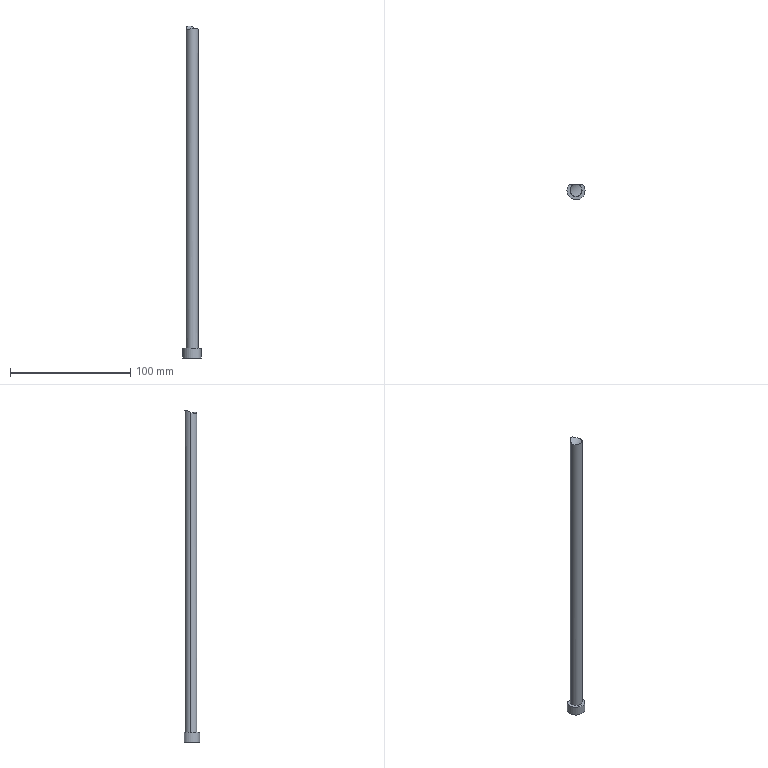Part | Creo | 1 solid | 7 faces | box 15 x 13 x 276.072 mm | volume 22178 mm3 | cylinder 4 | plane 3 | commonest cylinder face diameters 10 x2 15 x1 16.668 x1
STEP:
#1=CARTESIAN_POINT('',(0.,0.,0.));
#2=DIRECTION('',(0.,0.,1.));
#3=DIRECTION('',(1.,0.,0.));
#4=AXIS2_PLACEMENT_3D('',#1,#2,#3);
#5=CARTESIAN_POINT('',(243.229,48.9,-330.441));
#6=VERTEX_POINT('',#5);
#7=CARTESIAN_POINT('',(240.828,43.4,-330.441));
#8=VERTEX_POINT('',#7);
#9=CARTESIAN_POINT('',(248.328,43.4,-330.441));
#10=DIRECTION('',(0.,0.,1.));
#11=DIRECTION('',(-0.6799,0.7333,0.));
#12=AXIS2_PLACEMENT_3D('',#9,#10,#11);
#13=CIRCLE('',#12,7.5);
#14=EDGE_CURVE('',#6,#8,#13,.T.);
#15=ORIENTED_EDGE('',*,*,#14,.F.);
#16=CARTESIAN_POINT('',(253.427,48.9,-330.441));
#17=VERTEX_POINT('',#16);
#18=CARTESIAN_POINT('',(243.229,48.9,-330.441));
#19=DIRECTION('',(1.,0.,0.));
#20=VECTOR('',#19,10.198);
#21=LINE('',#18,#20);
#22=EDGE_CURVE('',#6,#17,#21,.T.);
#23=ORIENTED_EDGE('',*,*,#22,.T.);
#24=CARTESIAN_POINT('',(248.328,43.4,-330.441));
#25=DIRECTION('',(0.,0.,1.));
#26=DIRECTION('',(-1.,0.,0.));
#27=AXIS2_PLACEMENT_3D('',#24,#25,#26);
#28=CIRCLE('',#27,7.5);
#29=EDGE_CURVE('',#8,#17,#28,.T.);
#30=ORIENTED_EDGE('',*,*,#29,.F.);
#31=EDGE_LOOP('',(#15,#23,#30));
#32=FACE_OUTER_BOUND('',#31,.F.);
#33=CARTESIAN_POINT('',(253.328,43.4,-330.441));
#34=VERTEX_POINT('',#33);
#35=CARTESIAN_POINT('',(243.328,43.4,-330.441));
#36=VERTEX_POINT('',#35);
#37=CARTESIAN_POINT('',(248.328,43.4,-330.441));
#38=DIRECTION('',(0.,0.,-1.));
#39=DIRECTION('',(1.,0.,0.));
#40=AXIS2_PLACEMENT_3D('',#37,#38,#39);
#41=CIRCLE('',#40,5.);
#42=EDGE_CURVE('',#34,#36,#41,.T.);
#43=ORIENTED_EDGE('',*,*,#42,.F.);
#44=CARTESIAN_POINT('',(248.328,43.4,-330.441));
#45=DIRECTION('',(0.,0.,-1.));
#46=DIRECTION('',(-1.,0.,0.));
#47=AXIS2_PLACEMENT_3D('',#44,#45,#46);
#48=CIRCLE('',#47,5.);
#49=EDGE_CURVE('',#36,#34,#48,.T.);
#50=ORIENTED_EDGE('',*,*,#49,.F.);
#51=EDGE_LOOP('',(#43,#50));
#52=FACE_BOUND('',#51,.F.);
#53=CARTESIAN_POINT('',(248.328,43.4,-330.441));
#54=DIRECTION('',(0.,0.,1.));
#55=DIRECTION('',(1.,0.,0.));
#56=AXIS2_PLACEMENT_3D('',#53,#54,#55);
#57=PLANE('',#56);
#58=ADVANCED_FACE('',(#32,#52),#57,.T.);
#59=ORIENTED_EDGE('',*,*,#42,.T.);
#60=CARTESIAN_POINT('',(243.33,43.399,-64.325));
#61=VERTEX_POINT('',#60);
#62=CARTESIAN_POINT('',(243.328,43.4,-330.441));
#63=DIRECTION('',(0.000004071,-0.000003225,1.));
#64=VECTOR('',#63,266.117);
#65=LINE('',#62,#64);
#66=EDGE_CURVE('',#36,#61,#65,.T.);
#67=ORIENTED_EDGE('',*,*,#66,.T.);
#68=CARTESIAN_POINT('',(253.328,43.4,-65.042));
#69=VERTEX_POINT('',#68);
#70=CARTESIAN_POINT('',(243.33,43.399,-64.325));
#71=CARTESIAN_POINT('',(243.33,42.96,-64.508));
#72=CARTESIAN_POINT('',(243.442,42.11,-64.814));
#73=CARTESIAN_POINT('',(243.914,40.947,-65.081));
#74=CARTESIAN_POINT('',(244.639,39.95,-65.155));
#75=CARTESIAN_POINT('',(245.617,39.13,-65.057));
#76=CARTESIAN_POINT('',(246.86,38.554,-64.804));
#77=CARTESIAN_POINT('',(248.226,38.339,-64.495));
#78=CARTESIAN_POINT('',(249.568,38.496,-64.257));
#79=CARTESIAN_POINT('',(250.795,38.986,-64.177));
#80=CARTESIAN_POINT('',(251.838,39.76,-64.275));
#81=CARTESIAN_POINT('',(252.664,40.791,-64.515));
#82=CARTESIAN_POINT('',(253.204,42.044,-64.819));
#83=CARTESIAN_POINT('',(253.328,42.933,-64.984));
#84=CARTESIAN_POINT('',(253.328,43.4,-65.042));
#85=B_SPLINE_CURVE_WITH_KNOTS('',3,(#70,#71,#72,#73,#74,#75,#76,#77,#78,#79,#80,#81,#82,#83,#84),.UNSPECIFIED.,.F.,.F.,(4,1,1,1,1,1,1,1,1,1,1,1,4),(0.,0.08333,0.1667,0.25,0.3333,0.4167,0.5,0.5833,0.6667,0.75,0.8333,0.9167,1.),.UNSPECIFIED.);
#86=EDGE_CURVE('',#61,#69,#85,.T.);
#87=ORIENTED_EDGE('',*,*,#86,.T.);
#88=CARTESIAN_POINT('',(253.328,43.4,-330.441));
#89=DIRECTION('',(0.,0.,1.));
#90=VECTOR('',#89,265.399);
#91=LINE('',#88,#90);
#92=EDGE_CURVE('',#34,#69,#91,.T.);
#93=ORIENTED_EDGE('',*,*,#92,.F.);
#94=EDGE_LOOP('',(#59,#67,#87,#93));
#95=FACE_OUTER_BOUND('',#94,.F.);
#96=CARTESIAN_POINT('',(248.328,43.4,-653.441));
#97=DIRECTION('',(0.,0.,1.));
#98=DIRECTION('',(1.,0.,0.));
#99=AXIS2_PLACEMENT_3D('',#96,#97,#98);
#100=CYLINDRICAL_SURFACE('',#99,5.);
#101=ADVANCED_FACE('',(#95),#100,.T.);
#102=ORIENTED_EDGE('',*,*,#49,.T.);
#103=ORIENTED_EDGE('',*,*,#92,.T.);
#104=CARTESIAN_POINT('',(243.337,43.694,-64.198));
#105=VERTEX_POINT('',#104);
#106=CARTESIAN_POINT('',(253.328,43.4,-65.042));
#107=CARTESIAN_POINT('',(253.328,43.849,-65.099));
#108=CARTESIAN_POINT('',(253.21,44.72,-65.159));
#109=CARTESIAN_POINT('',(252.704,45.937,-65.054));
#110=CARTESIAN_POINT('',(251.887,46.998,-64.728));
#111=CARTESIAN_POINT('',(250.78,47.834,-64.184));
#112=CARTESIAN_POINT('',(249.434,48.344,-63.481));
#113=CARTESIAN_POINT('',(248.078,48.449,-62.837));
#114=CARTESIAN_POINT('',(246.872,48.23,-62.436));
#115=CARTESIAN_POINT('',(245.826,47.778,-62.323));
#116=CARTESIAN_POINT('',(244.898,47.097,-62.502));
#117=CARTESIAN_POINT('',(244.148,46.226,-62.92));
#118=CARTESIAN_POINT('',(243.575,45.125,-63.512));
#119=CARTESIAN_POINT('',(243.367,44.207,-63.972));
#120=B_SPLINE_CURVE_WITH_KNOTS('',3,(#106,#107,#108,#109,#110,#111,#112,#113,#114,#115,#116,#117,#118,#119,#104),.UNSPECIFIED.,.F.,.F.,(4,1,1,1,1,1,1,1,1,1,1,1,4),(0.,0.08333,0.1667,0.25,0.3333,0.4167,0.5,0.5833,0.6667,0.75,0.8333,0.9167,1.),.UNSPECIFIED.);
#121=EDGE_CURVE('',#69,#105,#120,.T.);
#122=ORIENTED_EDGE('',*,*,#121,.T.);
#123=CARTESIAN_POINT('',(243.337,43.694,-64.198));
#124=CARTESIAN_POINT('',(243.334,43.644,-64.22));
#125=CARTESIAN_POINT('',(243.329,43.544,-64.263));
#126=CARTESIAN_POINT('',(243.33,43.448,-64.304));
#127=CARTESIAN_POINT('',(243.33,43.399,-64.325));
#128=B_SPLINE_CURVE_WITH_KNOTS('',3,(#123,#124,#125,#126,#127),.UNSPECIFIED.,.F.,.F.,(4,1,4),(0.,0.5,1.),.UNSPECIFIED.);
#129=EDGE_CURVE('',#105,#61,#128,.T.);
#130=ORIENTED_EDGE('',*,*,#129,.T.);
#131=ORIENTED_EDGE('',*,*,#66,.F.);
#132=EDGE_LOOP('',(#102,#103,#122,#130,#131));
#133=FACE_OUTER_BOUND('',#132,.F.);
#134=CARTESIAN_POINT('',(248.328,43.4,-653.441));
#135=DIRECTION('',(0.,0.,1.));
#136=DIRECTION('',(1.,0.,0.));
#137=AXIS2_PLACEMENT_3D('',#134,#135,#136);
#138=CYLINDRICAL_SURFACE('',#137,5.);
#139=ADVANCED_FACE('',(#133),#138,.T.);
#140=ORIENTED_EDGE('',*,*,#86,.F.);
#141=ORIENTED_EDGE('',*,*,#129,.F.);
#142=ORIENTED_EDGE('',*,*,#121,.F.);
#143=EDGE_LOOP('',(#140,#141,#142));
#144=FACE_OUTER_BOUND('',#143,.F.);
#145=CARTESIAN_POINT('',(253.675,44.932,-56.793));
#146=DIRECTION('',(-0.8799,-0.4752,0.));
#147=DIRECTION('',(0.4752,-0.8799,0.));
#148=AXIS2_PLACEMENT_3D('',#145,#146,#147);
#149=CYLINDRICAL_SURFACE('',#148,8.334);
#150=ADVANCED_FACE('',(#144),#149,.F.);
#151=CARTESIAN_POINT('',(253.427,48.9,-338.441));
#152=VERTEX_POINT('',#151);
#153=CARTESIAN_POINT('',(253.427,48.9,-338.441));
#154=DIRECTION('',(0.,0.,1.));
#155=VECTOR('',#154,8.);
#156=LINE('',#153,#155);
#157=EDGE_CURVE('',#152,#17,#156,.T.);
#158=ORIENTED_EDGE('',*,*,#157,.F.);
#159=CARTESIAN_POINT('',(240.828,43.4,-338.441));
#160=VERTEX_POINT('',#159);
#161=CARTESIAN_POINT('',(248.328,43.4,-338.441));
#162=DIRECTION('',(0.,0.,-1.));
#163=DIRECTION('',(0.6799,0.7333,0.));
#164=AXIS2_PLACEMENT_3D('',#161,#162,#163);
#165=CIRCLE('',#164,7.5);
#166=EDGE_CURVE('',#152,#160,#165,.T.);
#167=ORIENTED_EDGE('',*,*,#166,.T.);
#168=CARTESIAN_POINT('',(243.229,48.9,-338.441));
#169=VERTEX_POINT('',#168);
#170=CARTESIAN_POINT('',(248.328,43.4,-338.441));
#171=DIRECTION('',(0.,0.,-1.));
#172=DIRECTION('',(-1.,0.,0.));
#173=AXIS2_PLACEMENT_3D('',#170,#171,#172);
#174=CIRCLE('',#173,7.5);
#175=EDGE_CURVE('',#160,#169,#174,.T.);
#176=ORIENTED_EDGE('',*,*,#175,.T.);
#177=CARTESIAN_POINT('',(243.229,48.9,-330.441));
#178=DIRECTION('',(0.,0.,-1.));
#179=VECTOR('',#178,8.);
#180=LINE('',#177,#179);
#181=EDGE_CURVE('',#6,#169,#180,.T.);
#182=ORIENTED_EDGE('',*,*,#181,.F.);
#183=ORIENTED_EDGE('',*,*,#14,.T.);
#184=ORIENTED_EDGE('',*,*,#29,.T.);
#185=EDGE_LOOP('',(#158,#167,#176,#182,#183,#184));
#186=FACE_OUTER_BOUND('',#185,.F.);
#187=CARTESIAN_POINT('',(248.328,43.4,-330.441));
#188=DIRECTION('',(0.,0.,-1.));
#189=DIRECTION('',(-1.,0.,0.));
#190=AXIS2_PLACEMENT_3D('',#187,#188,#189);
#191=CYLINDRICAL_SURFACE('',#190,7.5);
#192=ADVANCED_FACE('',(#186),#191,.T.);
#193=ORIENTED_EDGE('',*,*,#22,.F.);
#194=ORIENTED_EDGE('',*,*,#181,.T.);
#195=CARTESIAN_POINT('',(243.229,48.9,-338.441));
#196=DIRECTION('',(1.,0.,0.));
#197=VECTOR('',#196,10.198);
#198=LINE('',#195,#197);
#199=EDGE_CURVE('',#169,#152,#198,.T.);
#200=ORIENTED_EDGE('',*,*,#199,.T.);
#201=ORIENTED_EDGE('',*,*,#157,.T.);
#202=EDGE_LOOP('',(#193,#194,#200,#201));
#203=FACE_OUTER_BOUND('',#202,.F.);
#204=CARTESIAN_POINT('',(248.328,48.9,-338.441));
#205=DIRECTION('',(0.,1.,0.));
#206=DIRECTION('',(0.,0.,1.));
#207=AXIS2_PLACEMENT_3D('',#204,#205,#206);
#208=PLANE('',#207);
#209=ADVANCED_FACE('',(#203),#208,.T.);
#210=ORIENTED_EDGE('',*,*,#199,.F.);
#211=ORIENTED_EDGE('',*,*,#175,.F.);
#212=ORIENTED_EDGE('',*,*,#166,.F.);
#213=EDGE_LOOP('',(#210,#211,#212));
#214=FACE_OUTER_BOUND('',#213,.F.);
#215=CARTESIAN_POINT('',(248.328,43.4,-338.441));
#216=DIRECTION('',(0.,0.,1.));
#217=DIRECTION('',(1.,0.,0.));
#218=AXIS2_PLACEMENT_3D('',#215,#216,#217);
#219=PLANE('',#218);
#220=ADVANCED_FACE('',(#214),#219,.F.);
#221=CLOSED_SHELL('',(#58,#101,#139,#150,#192,#209,#220));
#222=MANIFOLD_SOLID_BREP('',#221);
#223=(LENGTH_UNIT()NAMED_UNIT(*)SI_UNIT(.MILLI.,.METRE.));
#224=UNCERTAINTY_MEASURE_WITH_UNIT(LENGTH_MEASURE(0.02768),#223,'','');
#225=(NAMED_UNIT(*)PLANE_ANGLE_UNIT()SI_UNIT($,.RADIAN.));
#226=PLANE_ANGLE_MEASURE_WITH_UNIT(PLANE_ANGLE_MEASURE(0.01745),#225);
#227=(CONVERSION_BASED_UNIT('DEGREE',#226)NAMED_UNIT(*)PLANE_ANGLE_UNIT());
#228=(NAMED_UNIT(*)SI_UNIT($,.STERADIAN.)SOLID_ANGLE_UNIT());
#229=(GEOMETRIC_REPRESENTATION_CONTEXT(3)GLOBAL_UNCERTAINTY_ASSIGNED_CONTEXT((#224))GLOBAL_UNIT_ASSIGNED_CONTEXT((#223,#227,#228))REPRESENTATION_CONTEXT('',''));
#230=ADVANCED_BREP_SHAPE_REPRESENTATION('',(#4,#222),#229);